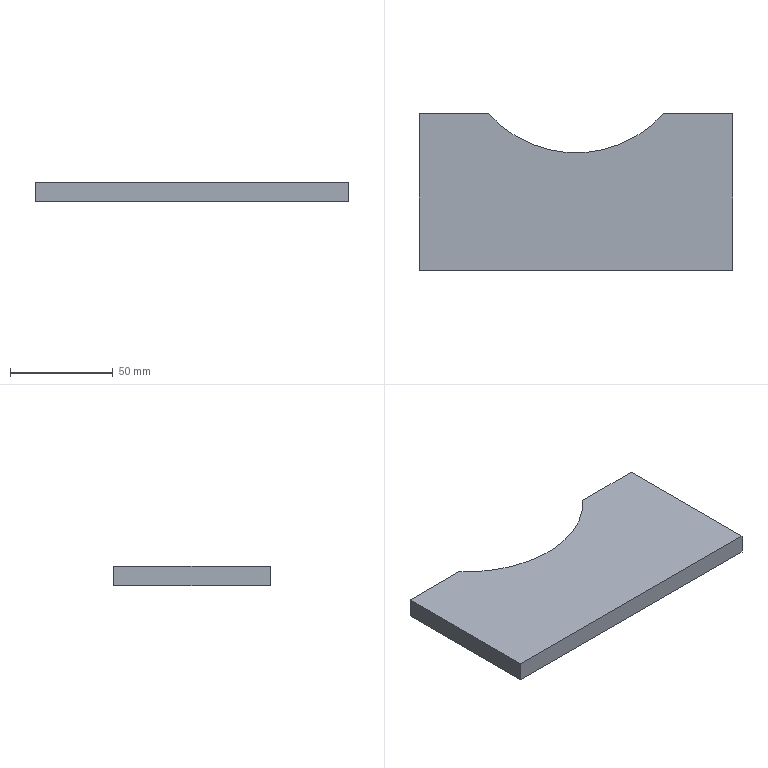Part | SolidWorks | features Extrusion 1 | 1 solid | 8 faces | box 152.4 x 76.2 x 9.525 mm | volume 99906 mm3 | plane 7 | cylinder 1 | commonest cylinder face diameters 114.3 x1
STEP:
#1=CARTESIAN_POINT('',(-76.2,-38.1,133.35));
#2=VERTEX_POINT('',#1);
#3=CARTESIAN_POINT('',(-76.2,-114.3,133.35));
#4=VERTEX_POINT('',#3);
#5=CARTESIAN_POINT('',(-76.2,-38.1,133.35));
#6=DIRECTION('',(0.,-1.,0.));
#7=VECTOR('',#6,1000.);
#8=LINE('',#5,#7);
#9=EDGE_CURVE('',#2,#4,#8,.T.);
#10=ORIENTED_EDGE('',*,*,#9,.F.);
#11=CARTESIAN_POINT('',(-76.2,-38.1,123.825));
#12=VERTEX_POINT('',#11);
#13=CARTESIAN_POINT('',(-76.2,-38.1,123.825));
#14=DIRECTION('',(0.,0.,1.));
#15=VECTOR('',#14,1000.);
#16=LINE('',#13,#15);
#17=EDGE_CURVE('',#12,#2,#16,.T.);
#18=ORIENTED_EDGE('',*,*,#17,.F.);
#19=CARTESIAN_POINT('',(-76.2,-114.3,123.825));
#20=VERTEX_POINT('',#19);
#21=CARTESIAN_POINT('',(-76.2,-38.1,123.825));
#22=DIRECTION('',(0.,-1.,0.));
#23=VECTOR('',#22,1000.);
#24=LINE('',#21,#23);
#25=EDGE_CURVE('',#12,#20,#24,.T.);
#26=ORIENTED_EDGE('',*,*,#25,.T.);
#27=CARTESIAN_POINT('',(-76.2,-114.3,123.825));
#28=DIRECTION('',(0.,0.,1.));
#29=VECTOR('',#28,1000.);
#30=LINE('',#27,#29);
#31=EDGE_CURVE('',#20,#4,#30,.T.);
#32=ORIENTED_EDGE('',*,*,#31,.T.);
#33=EDGE_LOOP('',(#10,#18,#26,#32));
#34=FACE_OUTER_BOUND('',#33,.T.);
#35=CARTESIAN_POINT('',(-76.2,-38.1,123.825));
#36=DIRECTION('',(-1.,0.,0.));
#37=DIRECTION('',(0.,-1.,0.));
#38=AXIS2_PLACEMENT_3D('',#35,#36,#37);
#39=PLANE('',#38);
#40=ADVANCED_FACE('',(#34),#39,.T.);
#41=CARTESIAN_POINT('',(-42.597,-38.1,133.35));
#42=VERTEX_POINT('',#41);
#43=CARTESIAN_POINT('',(-76.2,-38.1,133.35));
#44=DIRECTION('',(-1.,0.,0.));
#45=VECTOR('',#44,1000.);
#46=LINE('',#43,#45);
#47=EDGE_CURVE('',#42,#2,#46,.T.);
#48=ORIENTED_EDGE('',*,*,#47,.F.);
#49=CARTESIAN_POINT('',(-42.597,-38.1,123.825));
#50=VERTEX_POINT('',#49);
#51=CARTESIAN_POINT('',(-42.597,-38.1,123.825));
#52=DIRECTION('',(0.,0.,1.));
#53=VECTOR('',#52,1000.);
#54=LINE('',#51,#53);
#55=EDGE_CURVE('',#50,#42,#54,.T.);
#56=ORIENTED_EDGE('',*,*,#55,.F.);
#57=CARTESIAN_POINT('',(-76.2,-38.1,123.825));
#58=DIRECTION('',(-1.,0.,0.));
#59=VECTOR('',#58,1000.);
#60=LINE('',#57,#59);
#61=EDGE_CURVE('',#50,#12,#60,.T.);
#62=ORIENTED_EDGE('',*,*,#61,.T.);
#63=ORIENTED_EDGE('',*,*,#17,.T.);
#64=EDGE_LOOP('',(#48,#56,#62,#63));
#65=FACE_OUTER_BOUND('',#64,.T.);
#66=CARTESIAN_POINT('',(-76.2,-38.1,123.825));
#67=DIRECTION('',(0.,1.,0.));
#68=DIRECTION('',(-1.,0.,0.));
#69=AXIS2_PLACEMENT_3D('',#66,#67,#68);
#70=PLANE('',#69);
#71=ADVANCED_FACE('',(#65),#70,.T.);
#72=CARTESIAN_POINT('',(42.597,-38.1,133.35));
#73=VERTEX_POINT('',#72);
#74=CARTESIAN_POINT('',(0.,0.,133.35));
#75=DIRECTION('',(0.,0.,-1.));
#76=DIRECTION('',(1.,0.,0.));
#77=AXIS2_PLACEMENT_3D('',#74,#75,#76);
#78=CIRCLE('',#77,57.15);
#79=EDGE_CURVE('',#73,#42,#78,.T.);
#80=ORIENTED_EDGE('',*,*,#79,.F.);
#81=CARTESIAN_POINT('',(42.597,-38.1,123.825));
#82=VERTEX_POINT('',#81);
#83=CARTESIAN_POINT('',(42.597,-38.1,123.825));
#84=DIRECTION('',(0.,0.,1.));
#85=VECTOR('',#84,1000.);
#86=LINE('',#83,#85);
#87=EDGE_CURVE('',#82,#73,#86,.T.);
#88=ORIENTED_EDGE('',*,*,#87,.F.);
#89=CARTESIAN_POINT('',(0.,0.,123.825));
#90=DIRECTION('',(0.,0.,-1.));
#91=DIRECTION('',(1.,0.,0.));
#92=AXIS2_PLACEMENT_3D('',#89,#90,#91);
#93=CIRCLE('',#92,57.15);
#94=EDGE_CURVE('',#82,#50,#93,.T.);
#95=ORIENTED_EDGE('',*,*,#94,.T.);
#96=ORIENTED_EDGE('',*,*,#55,.T.);
#97=EDGE_LOOP('',(#80,#88,#95,#96));
#98=FACE_OUTER_BOUND('',#97,.T.);
#99=CARTESIAN_POINT('',(0.,0.,123.825));
#100=DIRECTION('',(0.,0.,1.));
#101=DIRECTION('',(1.,0.,0.));
#102=AXIS2_PLACEMENT_3D('',#99,#100,#101);
#103=CYLINDRICAL_SURFACE('',#102,57.15);
#104=ADVANCED_FACE('',(#98),#103,.F.);
#105=CARTESIAN_POINT('',(76.2,-38.1,133.35));
#106=VERTEX_POINT('',#105);
#107=CARTESIAN_POINT('',(42.597,-38.1,133.35));
#108=DIRECTION('',(-1.,0.,0.));
#109=VECTOR('',#108,1000.);
#110=LINE('',#107,#109);
#111=EDGE_CURVE('',#106,#73,#110,.T.);
#112=ORIENTED_EDGE('',*,*,#111,.F.);
#113=CARTESIAN_POINT('',(76.2,-38.1,123.825));
#114=VERTEX_POINT('',#113);
#115=CARTESIAN_POINT('',(76.2,-38.1,123.825));
#116=DIRECTION('',(0.,0.,1.));
#117=VECTOR('',#116,1000.);
#118=LINE('',#115,#117);
#119=EDGE_CURVE('',#114,#106,#118,.T.);
#120=ORIENTED_EDGE('',*,*,#119,.F.);
#121=CARTESIAN_POINT('',(42.597,-38.1,123.825));
#122=DIRECTION('',(-1.,0.,0.));
#123=VECTOR('',#122,1000.);
#124=LINE('',#121,#123);
#125=EDGE_CURVE('',#114,#82,#124,.T.);
#126=ORIENTED_EDGE('',*,*,#125,.T.);
#127=ORIENTED_EDGE('',*,*,#87,.T.);
#128=EDGE_LOOP('',(#112,#120,#126,#127));
#129=FACE_OUTER_BOUND('',#128,.T.);
#130=CARTESIAN_POINT('',(42.597,-38.1,123.825));
#131=DIRECTION('',(0.,1.,0.));
#132=DIRECTION('',(0.,0.,1.));
#133=AXIS2_PLACEMENT_3D('',#130,#131,#132);
#134=PLANE('',#133);
#135=ADVANCED_FACE('',(#129),#134,.T.);
#136=CARTESIAN_POINT('',(76.2,-114.3,133.35));
#137=VERTEX_POINT('',#136);
#138=CARTESIAN_POINT('',(76.2,-38.1,133.35));
#139=DIRECTION('',(0.,1.,0.));
#140=VECTOR('',#139,1000.);
#141=LINE('',#138,#140);
#142=EDGE_CURVE('',#137,#106,#141,.T.);
#143=ORIENTED_EDGE('',*,*,#142,.F.);
#144=CARTESIAN_POINT('',(76.2,-114.3,123.825));
#145=VERTEX_POINT('',#144);
#146=CARTESIAN_POINT('',(76.2,-114.3,123.825));
#147=DIRECTION('',(0.,0.,1.));
#148=VECTOR('',#147,1000.);
#149=LINE('',#146,#148);
#150=EDGE_CURVE('',#145,#137,#149,.T.);
#151=ORIENTED_EDGE('',*,*,#150,.F.);
#152=CARTESIAN_POINT('',(76.2,-38.1,123.825));
#153=DIRECTION('',(0.,1.,0.));
#154=VECTOR('',#153,1000.);
#155=LINE('',#152,#154);
#156=EDGE_CURVE('',#145,#114,#155,.T.);
#157=ORIENTED_EDGE('',*,*,#156,.T.);
#158=ORIENTED_EDGE('',*,*,#119,.T.);
#159=EDGE_LOOP('',(#143,#151,#157,#158));
#160=FACE_OUTER_BOUND('',#159,.T.);
#161=CARTESIAN_POINT('',(76.2,-38.1,123.825));
#162=DIRECTION('',(1.,0.,0.));
#163=DIRECTION('',(0.,1.,0.));
#164=AXIS2_PLACEMENT_3D('',#161,#162,#163);
#165=PLANE('',#164);
#166=ADVANCED_FACE('',(#160),#165,.T.);
#167=CARTESIAN_POINT('',(-76.2,-114.3,133.35));
#168=DIRECTION('',(1.,0.,0.));
#169=VECTOR('',#168,1000.);
#170=LINE('',#167,#169);
#171=EDGE_CURVE('',#4,#137,#170,.T.);
#172=ORIENTED_EDGE('',*,*,#171,.F.);
#173=ORIENTED_EDGE('',*,*,#31,.F.);
#174=CARTESIAN_POINT('',(-76.2,-114.3,123.825));
#175=DIRECTION('',(1.,0.,0.));
#176=VECTOR('',#175,1000.);
#177=LINE('',#174,#176);
#178=EDGE_CURVE('',#20,#145,#177,.T.);
#179=ORIENTED_EDGE('',*,*,#178,.T.);
#180=ORIENTED_EDGE('',*,*,#150,.T.);
#181=EDGE_LOOP('',(#172,#173,#179,#180));
#182=FACE_OUTER_BOUND('',#181,.T.);
#183=CARTESIAN_POINT('',(-76.2,-114.3,123.825));
#184=DIRECTION('',(0.,-1.,0.));
#185=DIRECTION('',(1.,0.,0.));
#186=AXIS2_PLACEMENT_3D('',#183,#184,#185);
#187=PLANE('',#186);
#188=ADVANCED_FACE('',(#182),#187,.T.);
#189=ORIENTED_EDGE('',*,*,#25,.F.);
#190=ORIENTED_EDGE('',*,*,#61,.F.);
#191=ORIENTED_EDGE('',*,*,#94,.F.);
#192=ORIENTED_EDGE('',*,*,#125,.F.);
#193=ORIENTED_EDGE('',*,*,#156,.F.);
#194=ORIENTED_EDGE('',*,*,#178,.F.);
#195=EDGE_LOOP('',(#189,#190,#191,#192,#193,#194));
#196=FACE_OUTER_BOUND('',#195,.T.);
#197=CARTESIAN_POINT('',(0.,0.,123.825));
#198=DIRECTION('',(0.,0.,1.));
#199=DIRECTION('',(1.,0.,0.));
#200=AXIS2_PLACEMENT_3D('',#197,#198,#199);
#201=PLANE('',#200);
#202=ADVANCED_FACE('',(#196),#201,.F.);
#203=ORIENTED_EDGE('',*,*,#9,.T.);
#204=ORIENTED_EDGE('',*,*,#171,.T.);
#205=ORIENTED_EDGE('',*,*,#142,.T.);
#206=ORIENTED_EDGE('',*,*,#111,.T.);
#207=ORIENTED_EDGE('',*,*,#79,.T.);
#208=ORIENTED_EDGE('',*,*,#47,.T.);
#209=EDGE_LOOP('',(#203,#204,#205,#206,#207,#208));
#210=FACE_OUTER_BOUND('',#209,.T.);
#211=CARTESIAN_POINT('',(0.,0.,133.35));
#212=DIRECTION('',(0.,0.,1.));
#213=DIRECTION('',(1.,0.,0.));
#214=AXIS2_PLACEMENT_3D('',#211,#212,#213);
#215=PLANE('',#214);
#216=ADVANCED_FACE('',(#210),#215,.T.);
#217=CLOSED_SHELL('',(#40,#71,#104,#135,#166,#188,#202,#216));
#218=MANIFOLD_SOLID_BREP('',#217);
#219=CARTESIAN_POINT('',(0.,0.,0.));
#220=DIRECTION('',(0.,0.,1.));
#221=DIRECTION('',(1.,0.,0.));
#222=AXIS2_PLACEMENT_3D('',#219,#220,#221);
#223=(LENGTH_UNIT()NAMED_UNIT(*)SI_UNIT(.MILLI.,.METRE.));
#224=UNCERTAINTY_MEASURE_WITH_UNIT(LENGTH_MEASURE(0.00001),#223,'','');
#225=(NAMED_UNIT(*)PLANE_ANGLE_UNIT()SI_UNIT($,.RADIAN.));
#226=(NAMED_UNIT(*)SI_UNIT($,.STERADIAN.)SOLID_ANGLE_UNIT());
#227=(GEOMETRIC_REPRESENTATION_CONTEXT(3)GLOBAL_UNCERTAINTY_ASSIGNED_CONTEXT((#224))GLOBAL_UNIT_ASSIGNED_CONTEXT((#223,#225,#226))REPRESENTATION_CONTEXT('',''));
#228=ADVANCED_BREP_SHAPE_REPRESENTATION('',(#218,#222),#227);